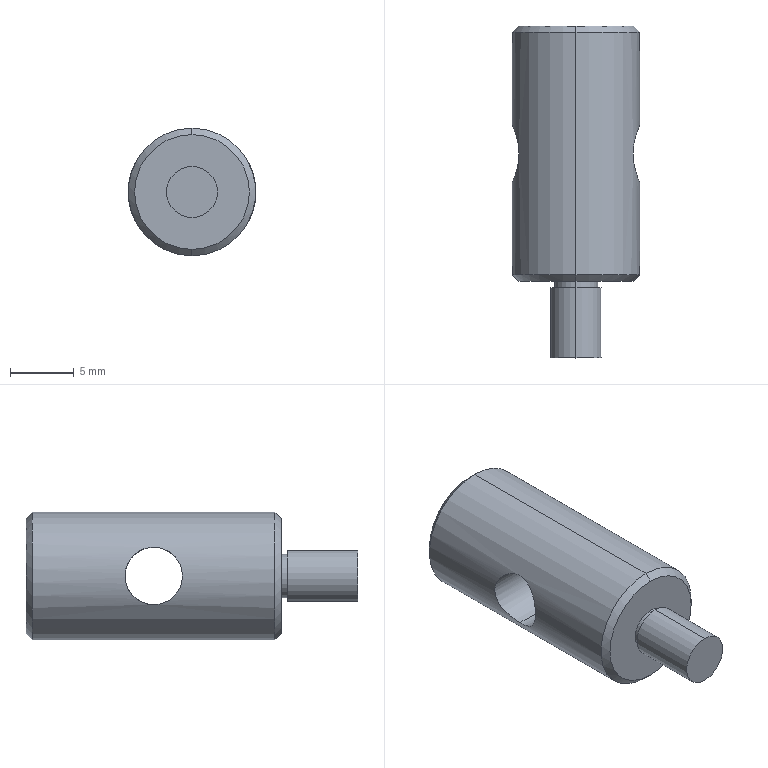Part | SolidWorks | features ICE 2, Chamfer 1, Extrusion 1, HoleWzd 1, RevCut 1 | 1 solid | 18 faces | box 10 x 26 x 10 mm | volume 1414 mm3 | cylinder 10 | cone 4 | plane 4 | commonest cylinder face diameters 3.3 x2 3.4 x2 4 x2 4.5 x2 10 x2
STEP:
#1=CARTESIAN_POINT('',(-4.465,0.,2.25));
#2=VERTEX_POINT('',#1);
#3=CARTESIAN_POINT('',(-4.465,0.,-2.25));
#4=VERTEX_POINT('',#3);
#5=CARTESIAN_POINT('',(-4.465,0.,2.25));
#6=CARTESIAN_POINT('',(-4.465,-0.2971,2.25));
#7=CARTESIAN_POINT('',(-4.497,-0.5965,2.189));
#8=CARTESIAN_POINT('',(-4.575,-1.004,2.019));
#9=CARTESIAN_POINT('',(-4.606,-1.134,1.949));
#10=CARTESIAN_POINT('',(-4.671,-1.376,1.786));
#11=CARTESIAN_POINT('',(-4.706,-1.488,1.694));
#12=CARTESIAN_POINT('',(-4.775,-1.695,1.487));
#13=CARTESIAN_POINT('',(-4.809,-1.787,1.374));
#14=CARTESIAN_POINT('',(-4.872,-1.949,1.133));
#15=CARTESIAN_POINT('',(-4.9,-2.02,1.003));
#16=CARTESIAN_POINT('',(-4.948,-2.134,0.7295));
#17=CARTESIAN_POINT('',(-4.967,-2.177,0.5887));
#18=CARTESIAN_POINT('',(-4.993,-2.235,0.2983));
#19=CARTESIAN_POINT('',(-5.,-2.25,0.1472));
#20=CARTESIAN_POINT('',(-5.,-2.25,-0.1543));
#21=CARTESIAN_POINT('',(-4.993,-2.235,-0.3021));
#22=CARTESIAN_POINT('',(-4.967,-2.176,-0.5924));
#23=CARTESIAN_POINT('',(-4.947,-2.131,-0.7362));
#24=CARTESIAN_POINT('',(-4.899,-2.017,-1.008));
#25=CARTESIAN_POINT('',(-4.871,-1.948,-1.136));
#26=CARTESIAN_POINT('',(-4.808,-1.784,-1.379));
#27=CARTESIAN_POINT('',(-4.773,-1.69,-1.492));
#28=CARTESIAN_POINT('',(-4.67,-1.383,-1.798));
#29=CARTESIAN_POINT('',(-4.6,-1.136,-1.964));
#30=CARTESIAN_POINT('',(-4.523,-0.7312,-2.133));
#31=CARTESIAN_POINT('',(-4.501,-0.5875,-2.177));
#32=CARTESIAN_POINT('',(-4.473,-0.2963,-2.235));
#33=CARTESIAN_POINT('',(-4.465,-0.149,-2.25));
#34=CARTESIAN_POINT('',(-4.465,0.,-2.25));
#35=B_SPLINE_CURVE_WITH_KNOTS('',3,(#5,#6,#7,#8,#9,#10,#11,#12,#13,#14,#15,#16,#17,#18,#19,#20,#21,#22,#23,#24,#25,#26,#27,#28,#29,#30,#31,#32,#33,#34),.UNSPECIFIED.,.F.,.F.,(4,2,2,2,2,2,2,2,2,2,2,2,2,2,4),(0.01069,0.01159,0.01203,0.01248,0.01292,0.01337,0.01381,0.01426,0.0147,0.01515,0.0156,0.01604,0.01693,0.01738,0.01782),.UNSPECIFIED.);
#36=EDGE_CURVE('',#2,#4,#35,.T.);
#37=ORIENTED_EDGE('',*,*,#36,.F.);
#38=CARTESIAN_POINT('',(4.465,0.,2.25));
#39=VERTEX_POINT('',#38);
#40=CARTESIAN_POINT('',(-5.,0.,2.25));
#41=DIRECTION('',(1.,0.,0.));
#42=VECTOR('',#41,1000.);
#43=LINE('',#40,#42);
#44=EDGE_CURVE('',#2,#39,#43,.T.);
#45=ORIENTED_EDGE('',*,*,#44,.T.);
#46=CARTESIAN_POINT('',(4.465,0.,-2.25));
#47=VERTEX_POINT('',#46);
#48=CARTESIAN_POINT('',(4.465,0.,-2.25));
#49=CARTESIAN_POINT('',(4.465,-0.1509,-2.25));
#50=CARTESIAN_POINT('',(4.473,-0.2988,-2.235));
#51=CARTESIAN_POINT('',(4.502,-0.589,-2.177));
#52=CARTESIAN_POINT('',(4.523,-0.7328,-2.132));
#53=CARTESIAN_POINT('',(4.601,-1.14,-1.962));
#54=CARTESIAN_POINT('',(4.671,-1.386,-1.796));
#55=CARTESIAN_POINT('',(4.809,-1.795,-1.387));
#56=CARTESIAN_POINT('',(4.876,-1.962,-1.139));
#57=CARTESIAN_POINT('',(4.948,-2.132,-0.7335));
#58=CARTESIAN_POINT('',(4.967,-2.176,-0.5896));
#59=CARTESIAN_POINT('',(4.993,-2.235,-0.298));
#60=CARTESIAN_POINT('',(5.,-2.25,-0.1505));
#61=CARTESIAN_POINT('',(5.,-2.25,0.1479));
#62=CARTESIAN_POINT('',(4.993,-2.235,0.299));
#63=CARTESIAN_POINT('',(4.967,-2.176,0.5897));
#64=CARTESIAN_POINT('',(4.948,-2.133,0.732));
#65=CARTESIAN_POINT('',(4.9,-2.018,1.006));
#66=CARTESIAN_POINT('',(4.871,-1.949,1.135));
#67=CARTESIAN_POINT('',(4.808,-1.786,1.377));
#68=CARTESIAN_POINT('',(4.774,-1.692,1.491));
#69=CARTESIAN_POINT('',(4.705,-1.486,1.695));
#70=CARTESIAN_POINT('',(4.67,-1.374,1.787));
#71=CARTESIAN_POINT('',(4.605,-1.131,1.95));
#72=CARTESIAN_POINT('',(4.574,-1.001,2.02));
#73=CARTESIAN_POINT('',(4.497,-0.5969,2.189));
#74=CARTESIAN_POINT('',(4.465,-0.2971,2.25));
#75=CARTESIAN_POINT('',(4.465,0.,2.25));
#76=B_SPLINE_CURVE_WITH_KNOTS('',3,(#48,#49,#50,#51,#52,#53,#54,#55,#56,#57,#58,#59,#60,#61,#62,#63,#64,#65,#66,#67,#68,#69,#70,#71,#72,#73,#74,#75),.UNSPECIFIED.,.F.,.F.,(4,2,2,2,2,2,2,2,2,2,2,2,2,4),(0.,0.0004457,0.0008914,0.001783,0.002674,0.00312,0.003566,0.004011,0.004457,0.004903,0.005348,0.005794,0.00624,0.007131),.UNSPECIFIED.);
#77=EDGE_CURVE('',#47,#39,#76,.T.);
#78=ORIENTED_EDGE('',*,*,#77,.F.);
#79=CARTESIAN_POINT('',(-5.,0.,-2.25));
#80=DIRECTION('',(1.,0.,0.));
#81=VECTOR('',#80,1000.);
#82=LINE('',#79,#81);
#83=EDGE_CURVE('',#4,#47,#82,.T.);
#84=ORIENTED_EDGE('',*,*,#83,.F.);
#85=EDGE_LOOP('',(#37,#45,#78,#84));
#86=FACE_OUTER_BOUND('',#85,.T.);
#87=CARTESIAN_POINT('',(-5.,0.,0.));
#88=DIRECTION('',(1.,0.,0.));
#89=DIRECTION('',(0.,0.,-1.));
#90=AXIS2_PLACEMENT_3D('',#87,#88,#89);
#91=CYLINDRICAL_SURFACE('',#90,2.25);
#92=ADVANCED_FACE('',(#86),#91,.F.);
#93=CARTESIAN_POINT('',(0.,-10.,-4.5));
#94=VERTEX_POINT('',#93);
#95=CARTESIAN_POINT('',(0.,-10.,4.5));
#96=VERTEX_POINT('',#95);
#97=CARTESIAN_POINT('',(0.,-10.,0.));
#98=DIRECTION('',(0.,-1.,0.));
#99=DIRECTION('',(0.,0.,1.));
#100=AXIS2_PLACEMENT_3D('',#97,#98,#99);
#101=CIRCLE('',#100,4.5);
#102=EDGE_CURVE('',#94,#96,#101,.T.);
#103=ORIENTED_EDGE('',*,*,#102,.F.);
#104=CARTESIAN_POINT('',(0.,-9.5,-5.));
#105=VERTEX_POINT('',#104);
#106=CARTESIAN_POINT('',(0.,-9.5,-5.));
#107=DIRECTION('',(0.,0.7071,-0.7071));
#108=VECTOR('',#107,1000.);
#109=LINE('',#106,#108);
#110=EDGE_CURVE('',#94,#105,#109,.T.);
#111=ORIENTED_EDGE('',*,*,#110,.T.);
#112=CARTESIAN_POINT('',(0.,-9.5,5.));
#113=VERTEX_POINT('',#112);
#114=CARTESIAN_POINT('',(0.,-9.5,0.));
#115=DIRECTION('',(0.,1.,0.));
#116=DIRECTION('',(0.,0.,1.));
#117=AXIS2_PLACEMENT_3D('',#114,#115,#116);
#118=CIRCLE('',#117,5.);
#119=EDGE_CURVE('',#113,#105,#118,.T.);
#120=ORIENTED_EDGE('',*,*,#119,.F.);
#121=CARTESIAN_POINT('',(0.,-9.5,5.));
#122=DIRECTION('',(0.,0.7071,0.7071));
#123=VECTOR('',#122,1000.);
#124=LINE('',#121,#123);
#125=EDGE_CURVE('',#96,#113,#124,.T.);
#126=ORIENTED_EDGE('',*,*,#125,.F.);
#127=EDGE_LOOP('',(#103,#111,#120,#126));
#128=FACE_OUTER_BOUND('',#127,.T.);
#129=CARTESIAN_POINT('',(0.,-9.5,0.));
#130=DIRECTION('',(0.,1.,0.));
#131=DIRECTION('',(0.,0.,1.));
#132=AXIS2_PLACEMENT_3D('',#129,#130,#131);
#133=CONICAL_SURFACE('',#132,5.,0.7854);
#134=ADVANCED_FACE('',(#128),#133,.T.);
#135=CARTESIAN_POINT('',(0.,10.,4.5));
#136=VERTEX_POINT('',#135);
#137=CARTESIAN_POINT('',(0.,10.,-4.5));
#138=VERTEX_POINT('',#137);
#139=CARTESIAN_POINT('',(0.,10.,0.));
#140=DIRECTION('',(0.,1.,0.));
#141=DIRECTION('',(0.,0.,1.));
#142=AXIS2_PLACEMENT_3D('',#139,#140,#141);
#143=CIRCLE('',#142,4.5);
#144=EDGE_CURVE('',#136,#138,#143,.T.);
#145=ORIENTED_EDGE('',*,*,#144,.F.);
#146=CARTESIAN_POINT('',(0.,9.5,5.));
#147=VERTEX_POINT('',#146);
#148=CARTESIAN_POINT('',(0.,10.,4.5));
#149=DIRECTION('',(0.,-0.7071,0.7071));
#150=VECTOR('',#149,1000.);
#151=LINE('',#148,#150);
#152=EDGE_CURVE('',#136,#147,#151,.T.);
#153=ORIENTED_EDGE('',*,*,#152,.T.);
#154=CARTESIAN_POINT('',(0.,9.5,-5.));
#155=VERTEX_POINT('',#154);
#156=CARTESIAN_POINT('',(0.,9.5,0.));
#157=DIRECTION('',(0.,-1.,0.));
#158=DIRECTION('',(0.,0.,1.));
#159=AXIS2_PLACEMENT_3D('',#156,#157,#158);
#160=CIRCLE('',#159,5.);
#161=EDGE_CURVE('',#155,#147,#160,.T.);
#162=ORIENTED_EDGE('',*,*,#161,.F.);
#163=CARTESIAN_POINT('',(0.,10.,-4.5));
#164=DIRECTION('',(0.,-0.7071,-0.7071));
#165=VECTOR('',#164,1000.);
#166=LINE('',#163,#165);
#167=EDGE_CURVE('',#138,#155,#166,.T.);
#168=ORIENTED_EDGE('',*,*,#167,.F.);
#169=EDGE_LOOP('',(#145,#153,#162,#168));
#170=FACE_OUTER_BOUND('',#169,.T.);
#171=CARTESIAN_POINT('',(0.,10.,0.));
#172=DIRECTION('',(0.,-1.,0.));
#173=DIRECTION('',(0.,0.,-1.));
#174=AXIS2_PLACEMENT_3D('',#171,#172,#173);
#175=CONICAL_SURFACE('',#174,4.5,0.7854);
#176=ADVANCED_FACE('',(#170),#175,.T.);
#177=CARTESIAN_POINT('',(0.,1.53,1.65));
#178=VERTEX_POINT('',#177);
#179=CARTESIAN_POINT('',(0.,1.53,-1.65));
#180=VERTEX_POINT('',#179);
#181=CARTESIAN_POINT('',(0.,1.53,1.65));
#182=CARTESIAN_POINT('',(-0.1143,1.53,1.65));
#183=CARTESIAN_POINT('',(-0.225,1.543,1.638));
#184=CARTESIAN_POINT('',(-0.4406,1.588,1.594));
#185=CARTESIAN_POINT('',(-0.5456,1.622,1.561));
#186=CARTESIAN_POINT('',(-0.8389,1.735,1.437));
#187=CARTESIAN_POINT('',(-1.012,1.831,1.319));
#188=CARTESIAN_POINT('',(-1.234,1.964,1.101));
#189=CARTESIAN_POINT('',(-1.302,2.008,1.02));
#190=CARTESIAN_POINT('',(-1.42,2.087,0.8466));
#191=CARTESIAN_POINT('',(-1.472,2.122,0.7541));
#192=CARTESIAN_POINT('',(-1.601,2.213,0.4552));
#193=CARTESIAN_POINT('',(-1.65,2.25,0.229));
#194=CARTESIAN_POINT('',(-1.65,2.25,-0.223));
#195=CARTESIAN_POINT('',(-1.603,2.215,-0.4478));
#196=CARTESIAN_POINT('',(-1.475,2.125,-0.7482));
#197=CARTESIAN_POINT('',(-1.422,2.088,-0.8435));
#198=CARTESIAN_POINT('',(-1.303,2.009,-1.018));
#199=CARTESIAN_POINT('',(-1.236,1.965,-1.099));
#200=CARTESIAN_POINT('',(-1.087,1.876,-1.245));
#201=CARTESIAN_POINT('',(-1.008,1.83,-1.311));
#202=CARTESIAN_POINT('',(-0.8358,1.742,-1.426));
#203=CARTESIAN_POINT('',(-0.7428,1.698,-1.477));
#204=CARTESIAN_POINT('',(-0.4488,1.584,-1.602));
#205=CARTESIAN_POINT('',(-0.2268,1.53,-1.65));
#206=CARTESIAN_POINT('',(0.,1.53,-1.65));
#207=B_SPLINE_CURVE_WITH_KNOTS('',3,(#181,#182,#183,#184,#185,#186,#187,#188,#189,#190,#191,#192,#193,#194,#195,#196,#197,#198,#199,#200,#201,#202,#203,#204,#205,#206),.UNSPECIFIED.,.F.,.F.,(4,2,2,2,2,2,2,2,2,2,2,2,4),(0.,0.000336,0.000672,0.001344,0.00168,0.002016,0.002688,0.00336,0.003696,0.004032,0.004368,0.004704,0.005376),.UNSPECIFIED.);
#208=EDGE_CURVE('',#178,#180,#207,.T.);
#209=ORIENTED_EDGE('',*,*,#208,.T.);
#210=CARTESIAN_POINT('',(0.,10.,-1.65));
#211=VERTEX_POINT('',#210);
#212=CARTESIAN_POINT('',(0.,10.,-1.65));
#213=DIRECTION('',(0.,1.,0.));
#214=VECTOR('',#213,1000.);
#215=LINE('',#212,#214);
#216=EDGE_CURVE('',#180,#211,#215,.T.);
#217=ORIENTED_EDGE('',*,*,#216,.T.);
#218=CARTESIAN_POINT('',(0.,10.,1.65));
#219=VERTEX_POINT('',#218);
#220=CARTESIAN_POINT('',(0.,10.,0.));
#221=DIRECTION('',(0.,1.,0.));
#222=DIRECTION('',(0.,0.,1.));
#223=AXIS2_PLACEMENT_3D('',#220,#221,#222);
#224=CIRCLE('',#223,1.65);
#225=EDGE_CURVE('',#211,#219,#224,.T.);
#226=ORIENTED_EDGE('',*,*,#225,.T.);
#227=CARTESIAN_POINT('',(0.,10.,1.65));
#228=DIRECTION('',(0.,1.,0.));
#229=VECTOR('',#228,1000.);
#230=LINE('',#227,#229);
#231=EDGE_CURVE('',#178,#219,#230,.T.);
#232=ORIENTED_EDGE('',*,*,#231,.F.);
#233=EDGE_LOOP('',(#209,#217,#226,#232));
#234=FACE_OUTER_BOUND('',#233,.T.);
#235=CARTESIAN_POINT('',(0.,10.,0.));
#236=DIRECTION('',(0.,1.,0.));
#237=DIRECTION('',(0.,0.,1.));
#238=AXIS2_PLACEMENT_3D('',#235,#236,#237);
#239=CYLINDRICAL_SURFACE('',#238,1.65);
#240=ADVANCED_FACE('',(#234),#239,.F.);
#241=CARTESIAN_POINT('',(0.,-16.,-2.));
#242=VERTEX_POINT('',#241);
#243=CARTESIAN_POINT('',(0.,-16.,2.));
#244=VERTEX_POINT('',#243);
#245=CARTESIAN_POINT('',(0.,-16.,0.));
#246=DIRECTION('',(0.,-1.,0.));
#247=DIRECTION('',(0.,0.,-1.));
#248=AXIS2_PLACEMENT_3D('',#245,#246,#247);
#249=CIRCLE('',#248,2.);
#250=EDGE_CURVE('',#242,#244,#249,.T.);
#251=ORIENTED_EDGE('',*,*,#250,.F.);
#252=CARTESIAN_POINT('',(0.,-10.5,-2.));
#253=VERTEX_POINT('',#252);
#254=CARTESIAN_POINT('',(0.,-16.,-2.));
#255=DIRECTION('',(0.,1.,0.));
#256=VECTOR('',#255,1000.);
#257=LINE('',#254,#256);
#258=EDGE_CURVE('',#242,#253,#257,.T.);
#259=ORIENTED_EDGE('',*,*,#258,.T.);
#260=CARTESIAN_POINT('',(0.,-10.5,2.));
#261=VERTEX_POINT('',#260);
#262=CARTESIAN_POINT('',(0.,-10.5,0.));
#263=DIRECTION('',(0.,1.,0.));
#264=DIRECTION('',(0.,0.,1.));
#265=AXIS2_PLACEMENT_3D('',#262,#263,#264);
#266=CIRCLE('',#265,2.);
#267=EDGE_CURVE('',#261,#253,#266,.T.);
#268=ORIENTED_EDGE('',*,*,#267,.F.);
#269=CARTESIAN_POINT('',(0.,-16.,2.));
#270=DIRECTION('',(0.,1.,0.));
#271=VECTOR('',#270,1000.);
#272=LINE('',#269,#271);
#273=EDGE_CURVE('',#244,#261,#272,.T.);
#274=ORIENTED_EDGE('',*,*,#273,.F.);
#275=EDGE_LOOP('',(#251,#259,#268,#274));
#276=FACE_OUTER_BOUND('',#275,.T.);
#277=CARTESIAN_POINT('',(0.,-16.,0.));
#278=DIRECTION('',(0.,1.,0.));
#279=DIRECTION('',(0.,0.,1.));
#280=AXIS2_PLACEMENT_3D('',#277,#278,#279);
#281=CYLINDRICAL_SURFACE('',#280,2.);
#282=ADVANCED_FACE('',(#276),#281,.T.);
#283=CARTESIAN_POINT('',(0.,-10.5,1.7));
#284=VERTEX_POINT('',#283);
#285=CARTESIAN_POINT('',(0.,-10.5,-1.7));
#286=VERTEX_POINT('',#285);
#287=CARTESIAN_POINT('',(0.,-10.5,0.));
#288=DIRECTION('',(0.,1.,0.));
#289=DIRECTION('',(0.,0.,1.));
#290=AXIS2_PLACEMENT_3D('',#287,#288,#289);
#291=CIRCLE('',#290,1.7);
#292=EDGE_CURVE('',#284,#286,#291,.T.);
#293=ORIENTED_EDGE('',*,*,#292,.T.);
#294=CARTESIAN_POINT('',(0.,-10.,-1.7));
#295=VERTEX_POINT('',#294);
#296=CARTESIAN_POINT('',(0.,0.,-1.7));
#297=DIRECTION('',(0.,1.,0.));
#298=VECTOR('',#297,1000.);
#299=LINE('',#296,#298);
#300=EDGE_CURVE('',#286,#295,#299,.T.);
#301=ORIENTED_EDGE('',*,*,#300,.T.);
#302=CARTESIAN_POINT('',(0.,-10.,1.7));
#303=VERTEX_POINT('',#302);
#304=CARTESIAN_POINT('',(0.,-10.,0.));
#305=DIRECTION('',(0.,1.,0.));
#306=DIRECTION('',(0.,0.,1.));
#307=AXIS2_PLACEMENT_3D('',#304,#305,#306);
#308=CIRCLE('',#307,1.7);
#309=EDGE_CURVE('',#303,#295,#308,.T.);
#310=ORIENTED_EDGE('',*,*,#309,.F.);
#311=CARTESIAN_POINT('',(0.,0.,1.7));
#312=DIRECTION('',(0.,1.,0.));
#313=VECTOR('',#312,1000.);
#314=LINE('',#311,#313);
#315=EDGE_CURVE('',#284,#303,#314,.T.);
#316=ORIENTED_EDGE('',*,*,#315,.F.);
#317=EDGE_LOOP('',(#293,#301,#310,#316));
#318=FACE_OUTER_BOUND('',#317,.T.);
#319=CARTESIAN_POINT('',(0.,0.,0.));
#320=DIRECTION('',(0.,1.,0.));
#321=DIRECTION('',(0.,0.,1.));
#322=AXIS2_PLACEMENT_3D('',#319,#320,#321);
#323=CYLINDRICAL_SURFACE('',#322,1.7);
#324=ADVANCED_FACE('',(#318),#323,.T.);
#325=ORIENTED_EDGE('',*,*,#77,.T.);
#326=CARTESIAN_POINT('',(4.465,0.,2.25));
#327=CARTESIAN_POINT('',(4.465,0.1484,2.25));
#328=CARTESIAN_POINT('',(4.473,0.2993,2.235));
#329=CARTESIAN_POINT('',(4.502,0.5907,2.176));
#330=CARTESIAN_POINT('',(4.523,0.7315,2.133));
#331=CARTESIAN_POINT('',(4.601,1.14,1.962));
#332=CARTESIAN_POINT('',(4.671,1.386,1.797));
#333=CARTESIAN_POINT('',(4.775,1.694,1.488));
#334=CARTESIAN_POINT('',(4.809,1.786,1.376));
#335=CARTESIAN_POINT('',(4.871,1.949,1.134));
#336=CARTESIAN_POINT('',(4.9,2.019,1.003));
#337=CARTESIAN_POINT('',(4.948,2.133,0.7323));
#338=CARTESIAN_POINT('',(4.967,2.176,0.5918));
#339=CARTESIAN_POINT('',(4.993,2.235,0.3001));
#340=CARTESIAN_POINT('',(5.,2.25,0.1494));
#341=CARTESIAN_POINT('',(5.,2.25,-0.2961));
#342=CARTESIAN_POINT('',(4.972,2.19,-0.5956));
#343=CARTESIAN_POINT('',(4.9,2.019,-1.003));
#344=CARTESIAN_POINT('',(4.871,1.949,-1.134));
#345=CARTESIAN_POINT('',(4.809,1.786,-1.376));
#346=CARTESIAN_POINT('',(4.775,1.694,-1.488));
#347=CARTESIAN_POINT('',(4.705,1.487,-1.695));
#348=CARTESIAN_POINT('',(4.67,1.374,-1.787));
#349=CARTESIAN_POINT('',(4.605,1.134,-1.949));
#350=CARTESIAN_POINT('',(4.575,1.004,-2.019));
#351=CARTESIAN_POINT('',(4.523,0.7316,-2.133));
#352=CARTESIAN_POINT('',(4.502,0.5912,-2.176));
#353=CARTESIAN_POINT('',(4.473,0.3015,-2.235));
#354=CARTESIAN_POINT('',(4.465,0.1507,-2.25));
#355=CARTESIAN_POINT('',(4.465,0.,-2.25));
#356=B_SPLINE_CURVE_WITH_KNOTS('',3,(#326,#327,#328,#329,#330,#331,#332,#333,#334,#335,#336,#337,#338,#339,#340,#341,#342,#343,#344,#345,#346,#347,#348,#349,#350,#351,#352,#353,#354,#355),.UNSPECIFIED.,.F.,.F.,(4,2,2,2,2,2,2,2,2,2,2,2,2,2,4),(0.007131,0.007576,0.008021,0.008912,0.009357,0.009802,0.01025,0.01069,0.01158,0.01203,0.01247,0.01292,0.01336,0.01381,0.01425),.UNSPECIFIED.);
#357=EDGE_CURVE('',#39,#47,#356,.T.);
#358=ORIENTED_EDGE('',*,*,#357,.T.);
#359=EDGE_LOOP('',(#325,#358));
#360=FACE_BOUND('',#359,.T.);
#361=ORIENTED_EDGE('',*,*,#161,.T.);
#362=CARTESIAN_POINT('',(0.,10.,5.));
#363=DIRECTION('',(0.,-1.,0.));
#364=VECTOR('',#363,1000.);
#365=LINE('',#362,#364);
#366=EDGE_CURVE('',#147,#113,#365,.T.);
#367=ORIENTED_EDGE('',*,*,#366,.T.);
#368=ORIENTED_EDGE('',*,*,#119,.T.);
#369=CARTESIAN_POINT('',(0.,10.,-5.));
#370=DIRECTION('',(0.,-1.,0.));
#371=VECTOR('',#370,1000.);
#372=LINE('',#369,#371);
#373=EDGE_CURVE('',#155,#105,#372,.T.);
#374=ORIENTED_EDGE('',*,*,#373,.F.);
#375=EDGE_LOOP('',(#361,#367,#368,#374));
#376=FACE_OUTER_BOUND('',#375,.T.);
#377=CARTESIAN_POINT('',(0.,10.,0.));
#378=DIRECTION('',(0.,-1.,0.));
#379=DIRECTION('',(0.,0.,-1.));
#380=AXIS2_PLACEMENT_3D('',#377,#378,#379);
#381=CYLINDRICAL_SURFACE('',#380,5.);
#382=ADVANCED_FACE('',(#360,#376),#381,.T.);
#383=CARTESIAN_POINT('',(0.,-10.,0.));
#384=DIRECTION('',(0.,-1.,0.));
#385=DIRECTION('',(0.,0.,1.));
#386=AXIS2_PLACEMENT_3D('',#383,#384,#385);
#387=CIRCLE('',#386,4.5);
#388=EDGE_CURVE('',#96,#94,#387,.T.);
#389=ORIENTED_EDGE('',*,*,#388,.T.);
#390=ORIENTED_EDGE('',*,*,#102,.T.);
#391=EDGE_LOOP('',(#389,#390));
#392=FACE_OUTER_BOUND('',#391,.T.);
#393=ORIENTED_EDGE('',*,*,#309,.T.);
#394=CARTESIAN_POINT('',(0.,-10.,0.));
#395=DIRECTION('',(0.,1.,0.));
#396=DIRECTION('',(0.,0.,1.));
#397=AXIS2_PLACEMENT_3D('',#394,#395,#396);
#398=CIRCLE('',#397,1.7);
#399=EDGE_CURVE('',#295,#303,#398,.T.);
#400=ORIENTED_EDGE('',*,*,#399,.T.);
#401=EDGE_LOOP('',(#393,#400));
#402=FACE_BOUND('',#401,.T.);
#403=CARTESIAN_POINT('',(0.,-10.,0.));
#404=DIRECTION('',(0.,1.,0.));
#405=DIRECTION('',(0.,0.,1.));
#406=AXIS2_PLACEMENT_3D('',#403,#404,#405);
#407=PLANE('',#406);
#408=ADVANCED_FACE('',(#392,#402),#407,.F.);
#409=ORIENTED_EDGE('',*,*,#366,.F.);
#410=CARTESIAN_POINT('',(0.,9.5,0.));
#411=DIRECTION('',(0.,-1.,0.));
#412=DIRECTION('',(0.,0.,1.));
#413=AXIS2_PLACEMENT_3D('',#410,#411,#412);
#414=CIRCLE('',#413,5.);
#415=EDGE_CURVE('',#147,#155,#414,.T.);
#416=ORIENTED_EDGE('',*,*,#415,.T.);
#417=ORIENTED_EDGE('',*,*,#373,.T.);
#418=CARTESIAN_POINT('',(0.,-9.5,0.));
#419=DIRECTION('',(0.,1.,0.));
#420=DIRECTION('',(0.,0.,1.));
#421=AXIS2_PLACEMENT_3D('',#418,#419,#420);
#422=CIRCLE('',#421,5.);
#423=EDGE_CURVE('',#105,#113,#422,.T.);
#424=ORIENTED_EDGE('',*,*,#423,.T.);
#425=EDGE_LOOP('',(#409,#416,#417,#424));
#426=FACE_OUTER_BOUND('',#425,.T.);
#427=CARTESIAN_POINT('',(-4.465,0.,-2.25));
#428=CARTESIAN_POINT('',(-4.465,0.149,-2.25));
#429=CARTESIAN_POINT('',(-4.473,0.3001,-2.235));
#430=CARTESIAN_POINT('',(-4.502,0.5905,-2.176));
#431=CARTESIAN_POINT('',(-4.523,0.7325,-2.133));
#432=CARTESIAN_POINT('',(-4.575,1.005,-2.018));
#433=CARTESIAN_POINT('',(-4.605,1.134,-1.949));
#434=CARTESIAN_POINT('',(-4.671,1.375,-1.787));
#435=CARTESIAN_POINT('',(-4.706,1.489,-1.693));
#436=CARTESIAN_POINT('',(-4.775,1.694,-1.488));
#437=CARTESIAN_POINT('',(-4.809,1.786,-1.376));
#438=CARTESIAN_POINT('',(-4.872,1.95,-1.133));
#439=CARTESIAN_POINT('',(-4.9,2.02,-1.003));
#440=CARTESIAN_POINT('',(-4.972,2.189,-0.5975));
#441=CARTESIAN_POINT('',(-5.,2.25,-0.2977));
#442=CARTESIAN_POINT('',(-5.,2.25,0.148));
#443=CARTESIAN_POINT('',(-4.993,2.235,0.2991));
#444=CARTESIAN_POINT('',(-4.967,2.176,0.5907));
#445=CARTESIAN_POINT('',(-4.948,2.133,0.7318));
#446=CARTESIAN_POINT('',(-4.876,1.961,1.141));
#447=CARTESIAN_POINT('',(-4.809,1.795,1.387));
#448=CARTESIAN_POINT('',(-4.705,1.486,1.696));
#449=CARTESIAN_POINT('',(-4.67,1.374,1.788));
#450=CARTESIAN_POINT('',(-4.605,1.133,1.95));
#451=CARTESIAN_POINT('',(-4.574,1.002,2.02));
#452=CARTESIAN_POINT('',(-4.523,0.7312,2.133));
#453=CARTESIAN_POINT('',(-4.502,0.5909,2.176));
#454=CARTESIAN_POINT('',(-4.473,0.2994,2.235));
#455=CARTESIAN_POINT('',(-4.465,0.1485,2.25));
#456=CARTESIAN_POINT('',(-4.465,0.,2.25));
#457=B_SPLINE_CURVE_WITH_KNOTS('',3,(#427,#428,#429,#430,#431,#432,#433,#434,#435,#436,#437,#438,#439,#440,#441,#442,#443,#444,#445,#446,#447,#448,#449,#450,#451,#452,#453,#454,#455,#456),.UNSPECIFIED.,.F.,.F.,(4,2,2,2,2,2,2,2,2,2,2,2,2,2,4),(0.003568,0.004013,0.004458,0.004904,0.005349,0.005795,0.00624,0.007131,0.007577,0.008022,0.008913,0.009358,0.009804,0.01025,0.01069),.UNSPECIFIED.);
#458=EDGE_CURVE('',#4,#2,#457,.T.);
#459=ORIENTED_EDGE('',*,*,#458,.T.);
#460=ORIENTED_EDGE('',*,*,#36,.T.);
#461=EDGE_LOOP('',(#459,#460));
#462=FACE_BOUND('',#461,.T.);
#463=CARTESIAN_POINT('',(0.,10.,0.));
#464=DIRECTION('',(0.,-1.,0.));
#465=DIRECTION('',(0.,0.,-1.));
#466=AXIS2_PLACEMENT_3D('',#463,#464,#465);
#467=CYLINDRICAL_SURFACE('',#466,5.);
#468=ADVANCED_FACE('',(#426,#462),#467,.T.);
#469=CARTESIAN_POINT('',(0.,10.,0.));
#470=DIRECTION('',(0.,1.,0.));
#471=DIRECTION('',(0.,0.,1.));
#472=AXIS2_PLACEMENT_3D('',#469,#470,#471);
#473=CIRCLE('',#472,4.5);
#474=EDGE_CURVE('',#138,#136,#473,.T.);
#475=ORIENTED_EDGE('',*,*,#474,.T.);
#476=ORIENTED_EDGE('',*,*,#144,.T.);
#477=EDGE_LOOP('',(#475,#476));
#478=FACE_OUTER_BOUND('',#477,.T.);
#479=CARTESIAN_POINT('',(0.,10.,0.));
#480=DIRECTION('',(0.,1.,0.));
#481=DIRECTION('',(0.,0.,1.));
#482=AXIS2_PLACEMENT_3D('',#479,#480,#481);
#483=CIRCLE('',#482,1.65);
#484=EDGE_CURVE('',#219,#211,#483,.T.);
#485=ORIENTED_EDGE('',*,*,#484,.F.);
#486=ORIENTED_EDGE('',*,*,#225,.F.);
#487=EDGE_LOOP('',(#485,#486));
#488=FACE_BOUND('',#487,.T.);
#489=CARTESIAN_POINT('',(0.,10.,0.));
#490=DIRECTION('',(0.,1.,0.));
#491=DIRECTION('',(0.,0.,1.));
#492=AXIS2_PLACEMENT_3D('',#489,#490,#491);
#493=PLANE('',#492);
#494=ADVANCED_FACE('',(#478,#488),#493,.T.);
#495=ORIENTED_EDGE('',*,*,#300,.F.);
#496=CARTESIAN_POINT('',(0.,-10.5,0.));
#497=DIRECTION('',(0.,1.,0.));
#498=DIRECTION('',(0.,0.,1.));
#499=AXIS2_PLACEMENT_3D('',#496,#497,#498);
#500=CIRCLE('',#499,1.7);
#501=EDGE_CURVE('',#286,#284,#500,.T.);
#502=ORIENTED_EDGE('',*,*,#501,.T.);
#503=ORIENTED_EDGE('',*,*,#315,.T.);
#504=ORIENTED_EDGE('',*,*,#399,.F.);
#505=EDGE_LOOP('',(#495,#502,#503,#504));
#506=FACE_OUTER_BOUND('',#505,.T.);
#507=CARTESIAN_POINT('',(0.,0.,0.));
#508=DIRECTION('',(0.,1.,0.));
#509=DIRECTION('',(0.,0.,1.));
#510=AXIS2_PLACEMENT_3D('',#507,#508,#509);
#511=CYLINDRICAL_SURFACE('',#510,1.7);
#512=ADVANCED_FACE('',(#506),#511,.T.);
#513=ORIENTED_EDGE('',*,*,#267,.T.);
#514=CARTESIAN_POINT('',(0.,-10.5,0.));
#515=DIRECTION('',(0.,1.,0.));
#516=DIRECTION('',(0.,0.,1.));
#517=AXIS2_PLACEMENT_3D('',#514,#515,#516);
#518=CIRCLE('',#517,2.);
#519=EDGE_CURVE('',#253,#261,#518,.T.);
#520=ORIENTED_EDGE('',*,*,#519,.T.);
#521=EDGE_LOOP('',(#513,#520));
#522=FACE_OUTER_BOUND('',#521,.T.);
#523=ORIENTED_EDGE('',*,*,#292,.F.);
#524=ORIENTED_EDGE('',*,*,#501,.F.);
#525=EDGE_LOOP('',(#523,#524));
#526=FACE_BOUND('',#525,.T.);
#527=CARTESIAN_POINT('',(1.7,-10.5,0.));
#528=DIRECTION('',(0.,1.,0.));
#529=DIRECTION('',(0.,0.,1.));
#530=AXIS2_PLACEMENT_3D('',#527,#528,#529);
#531=PLANE('',#530);
#532=ADVANCED_FACE('',(#522,#526),#531,.T.);
#533=CARTESIAN_POINT('',(0.,-16.,0.));
#534=DIRECTION('',(0.,-1.,0.));
#535=DIRECTION('',(0.,0.,-1.));
#536=AXIS2_PLACEMENT_3D('',#533,#534,#535);
#537=CIRCLE('',#536,2.);
#538=EDGE_CURVE('',#244,#242,#537,.T.);
#539=ORIENTED_EDGE('',*,*,#538,.T.);
#540=ORIENTED_EDGE('',*,*,#250,.T.);
#541=EDGE_LOOP('',(#539,#540));
#542=FACE_OUTER_BOUND('',#541,.T.);
#543=CARTESIAN_POINT('',(0.,-16.,0.));
#544=DIRECTION('',(0.,-1.,0.));
#545=DIRECTION('',(0.,0.,-1.));
#546=AXIS2_PLACEMENT_3D('',#543,#544,#545);
#547=PLANE('',#546);
#548=ADVANCED_FACE('',(#542),#547,.T.);
#549=ORIENTED_EDGE('',*,*,#258,.F.);
#550=ORIENTED_EDGE('',*,*,#538,.F.);
#551=ORIENTED_EDGE('',*,*,#273,.T.);
#552=ORIENTED_EDGE('',*,*,#519,.F.);
#553=EDGE_LOOP('',(#549,#550,#551,#552));
#554=FACE_OUTER_BOUND('',#553,.T.);
#555=CARTESIAN_POINT('',(0.,-16.,0.));
#556=DIRECTION('',(0.,1.,0.));
#557=DIRECTION('',(0.,0.,1.));
#558=AXIS2_PLACEMENT_3D('',#555,#556,#557);
#559=CYLINDRICAL_SURFACE('',#558,2.);
#560=ADVANCED_FACE('',(#554),#559,.T.);
#561=ORIENTED_EDGE('',*,*,#216,.F.);
#562=CARTESIAN_POINT('',(0.,1.53,-1.65));
#563=CARTESIAN_POINT('',(0.2264,1.53,-1.65));
#564=CARTESIAN_POINT('',(0.4503,1.584,-1.601));
#565=CARTESIAN_POINT('',(0.8399,1.736,-1.436));
#566=CARTESIAN_POINT('',(1.014,1.831,-1.318));
#567=CARTESIAN_POINT('',(1.234,1.965,-1.1));
#568=CARTESIAN_POINT('',(1.302,2.008,-1.019));
#569=CARTESIAN_POINT('',(1.421,2.088,-0.8448));
#570=CARTESIAN_POINT('',(1.473,2.123,-0.7517));
#571=CARTESIAN_POINT('',(1.602,2.214,-0.4517));
#572=CARTESIAN_POINT('',(1.65,2.25,-0.23));
#573=CARTESIAN_POINT('',(1.65,2.25,0.1108));
#574=CARTESIAN_POINT('',(1.639,2.242,0.2223));
#575=CARTESIAN_POINT('',(1.594,2.209,0.4413));
#576=CARTESIAN_POINT('',(1.56,2.185,0.5482));
#577=CARTESIAN_POINT('',(1.475,2.125,0.748));
#578=CARTESIAN_POINT('',(1.422,2.088,0.8432));
#579=CARTESIAN_POINT('',(1.303,2.009,1.018));
#580=CARTESIAN_POINT('',(1.236,1.966,1.098));
#581=CARTESIAN_POINT('',(1.014,1.832,1.318));
#582=CARTESIAN_POINT('',(0.8435,1.737,1.434));
#583=CARTESIAN_POINT('',(0.5477,1.622,1.56));
#584=CARTESIAN_POINT('',(0.4448,1.59,1.593));
#585=CARTESIAN_POINT('',(0.2279,1.543,1.638));
#586=CARTESIAN_POINT('',(0.1141,1.53,1.65));
#587=CARTESIAN_POINT('',(0.,1.53,1.65));
#588=B_SPLINE_CURVE_WITH_KNOTS('',3,(#562,#563,#564,#565,#566,#567,#568,#569,#570,#571,#572,#573,#574,#575,#576,#577,#578,#579,#580,#581,#582,#583,#584,#585,#586,#587),.UNSPECIFIED.,.F.,.F.,(4,2,2,2,2,2,2,2,2,2,2,2,4),(0.005376,0.006047,0.006718,0.007053,0.007388,0.008059,0.008395,0.00873,0.009066,0.009401,0.01007,0.01041,0.01074),.UNSPECIFIED.);
#589=EDGE_CURVE('',#180,#178,#588,.T.);
#590=ORIENTED_EDGE('',*,*,#589,.T.);
#591=ORIENTED_EDGE('',*,*,#231,.T.);
#592=ORIENTED_EDGE('',*,*,#484,.T.);
#593=EDGE_LOOP('',(#561,#590,#591,#592));
#594=FACE_OUTER_BOUND('',#593,.T.);
#595=CARTESIAN_POINT('',(0.,10.,0.));
#596=DIRECTION('',(0.,1.,0.));
#597=DIRECTION('',(0.,0.,1.));
#598=AXIS2_PLACEMENT_3D('',#595,#596,#597);
#599=CYLINDRICAL_SURFACE('',#598,1.65);
#600=ADVANCED_FACE('',(#594),#599,.F.);
#601=ORIENTED_EDGE('',*,*,#152,.F.);
#602=ORIENTED_EDGE('',*,*,#474,.F.);
#603=ORIENTED_EDGE('',*,*,#167,.T.);
#604=ORIENTED_EDGE('',*,*,#415,.F.);
#605=EDGE_LOOP('',(#601,#602,#603,#604));
#606=FACE_OUTER_BOUND('',#605,.T.);
#607=CARTESIAN_POINT('',(0.,10.,0.));
#608=DIRECTION('',(0.,-1.,0.));
#609=DIRECTION('',(0.,0.,-1.));
#610=AXIS2_PLACEMENT_3D('',#607,#608,#609);
#611=CONICAL_SURFACE('',#610,4.5,0.7854);
#612=ADVANCED_FACE('',(#606),#611,.T.);
#613=ORIENTED_EDGE('',*,*,#110,.F.);
#614=ORIENTED_EDGE('',*,*,#388,.F.);
#615=ORIENTED_EDGE('',*,*,#125,.T.);
#616=ORIENTED_EDGE('',*,*,#423,.F.);
#617=EDGE_LOOP('',(#613,#614,#615,#616));
#618=FACE_OUTER_BOUND('',#617,.T.);
#619=CARTESIAN_POINT('',(0.,-9.5,0.));
#620=DIRECTION('',(0.,1.,0.));
#621=DIRECTION('',(0.,0.,1.));
#622=AXIS2_PLACEMENT_3D('',#619,#620,#621);
#623=CONICAL_SURFACE('',#622,5.,0.7854);
#624=ADVANCED_FACE('',(#618),#623,.T.);
#625=ORIENTED_EDGE('',*,*,#44,.F.);
#626=ORIENTED_EDGE('',*,*,#458,.F.);
#627=ORIENTED_EDGE('',*,*,#83,.T.);
#628=ORIENTED_EDGE('',*,*,#357,.F.);
#629=EDGE_LOOP('',(#625,#626,#627,#628));
#630=FACE_OUTER_BOUND('',#629,.T.);
#631=ORIENTED_EDGE('',*,*,#208,.F.);
#632=ORIENTED_EDGE('',*,*,#589,.F.);
#633=EDGE_LOOP('',(#631,#632));
#634=FACE_BOUND('',#633,.T.);
#635=CARTESIAN_POINT('',(-5.,0.,0.));
#636=DIRECTION('',(1.,0.,0.));
#637=DIRECTION('',(0.,0.,-1.));
#638=AXIS2_PLACEMENT_3D('',#635,#636,#637);
#639=CYLINDRICAL_SURFACE('',#638,2.25);
#640=ADVANCED_FACE('',(#630,#634),#639,.F.);
#641=CLOSED_SHELL('',(#92,#134,#176,#240,#282,#324,#382,#408,#468,#494,#512,#532,#548,#560,#600,#612,#624,#640));
#642=MANIFOLD_SOLID_BREP('',#641);
#643=CARTESIAN_POINT('',(0.,0.,0.));
#644=DIRECTION('',(0.,0.,1.));
#645=DIRECTION('',(1.,0.,0.));
#646=AXIS2_PLACEMENT_3D('',#643,#644,#645);
#647=(LENGTH_UNIT()NAMED_UNIT(*)SI_UNIT(.MILLI.,.METRE.));
#648=UNCERTAINTY_MEASURE_WITH_UNIT(LENGTH_MEASURE(0.00001),#647,'','');
#649=(NAMED_UNIT(*)PLANE_ANGLE_UNIT()SI_UNIT($,.RADIAN.));
#650=(NAMED_UNIT(*)SI_UNIT($,.STERADIAN.)SOLID_ANGLE_UNIT());
#651=(GEOMETRIC_REPRESENTATION_CONTEXT(3)GLOBAL_UNCERTAINTY_ASSIGNED_CONTEXT((#648))GLOBAL_UNIT_ASSIGNED_CONTEXT((#647,#649,#650))REPRESENTATION_CONTEXT('',''));
#652=ADVANCED_BREP_SHAPE_REPRESENTATION('',(#642,#646),#651);